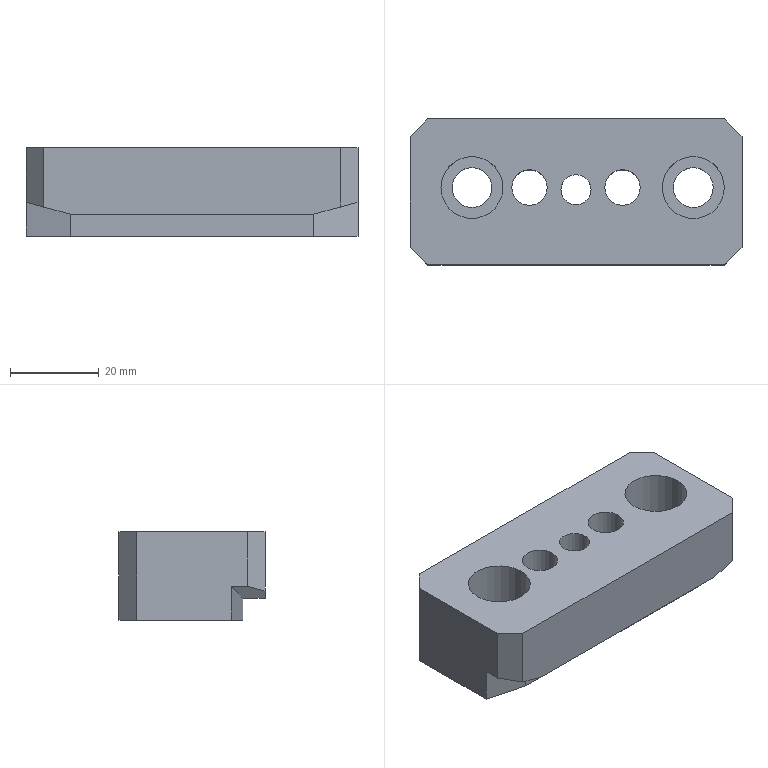Part | NX | features 20 2 | 1 solid | 25 faces | box 75 x 33 x 20 mm | volume 39698 mm3 | plane 18 | cylinder 7 | commonest cylinder face diameters 8.001 x2 9 x2 14 x2 6.8 x1
STEP:
#1=CARTESIAN_POINT('',(1899.002,435.,-3.5));
#2=VERTEX_POINT('',#1);
#3=CARTESIAN_POINT('',(1894.502,435.,-3.5));
#4=DIRECTION('',(0.,0.,-1.));
#5=DIRECTION('',(1.,0.,0.));
#6=AXIS2_PLACEMENT_3D('',#3,#4,#5);
#7=CIRCLE('',#6,4.5);
#8=EDGE_CURVE('',#2,#2,#7,.T.);
#9=ORIENTED_EDGE('',*,*,#8,.F.);
#10=EDGE_LOOP('',(#9));
#11=FACE_BOUND('',#10,.T.);
#12=CARTESIAN_POINT('',(1871.402,434.5,-3.5));
#13=VERTEX_POINT('',#12);
#14=CARTESIAN_POINT('',(1868.002,434.5,-3.5));
#15=DIRECTION('',(0.,0.,-1.));
#16=DIRECTION('',(1.,0.,0.));
#17=AXIS2_PLACEMENT_3D('',#14,#15,#16);
#18=CIRCLE('',#17,3.4);
#19=EDGE_CURVE('',#13,#13,#18,.T.);
#20=ORIENTED_EDGE('',*,*,#19,.F.);
#21=EDGE_LOOP('',(#20));
#22=FACE_BOUND('',#21,.T.);
#23=CARTESIAN_POINT('',(1849.002,435.,-3.5));
#24=VERTEX_POINT('',#23);
#25=CARTESIAN_POINT('',(1844.502,435.,-3.5));
#26=DIRECTION('',(0.,0.,1.));
#27=DIRECTION('',(1.,0.,0.));
#28=AXIS2_PLACEMENT_3D('',#25,#26,#27);
#29=CIRCLE('',#28,4.5);
#30=EDGE_CURVE('',#24,#24,#29,.T.);
#31=ORIENTED_EDGE('',*,*,#30,.T.);
#32=EDGE_LOOP('',(#31));
#33=FACE_BOUND('',#32,.T.);
#34=CARTESIAN_POINT('',(1895.501,422.5,-3.5));
#35=VERTEX_POINT('',#34);
#36=CARTESIAN_POINT('',(1840.501,422.5,-3.5));
#37=VERTEX_POINT('',#36);
#38=CARTESIAN_POINT('',(1906.501,422.5,-3.5));
#39=DIRECTION('',(-1.,0.,0.));
#40=VECTOR('',#39,1000.);
#41=LINE('',#38,#40);
#42=EDGE_CURVE('',#35,#37,#41,.T.);
#43=ORIENTED_EDGE('',*,*,#42,.T.);
#44=CARTESIAN_POINT('',(1830.502,425.179,-3.5));
#45=VERTEX_POINT('',#44);
#46=CARTESIAN_POINT('',(1840.501,422.5,-3.5));
#47=DIRECTION('',(-0.9659,0.2588,0.));
#48=VECTOR('',#47,1000.);
#49=LINE('',#46,#48);
#50=EDGE_CURVE('',#37,#45,#49,.T.);
#51=ORIENTED_EDGE('',*,*,#50,.T.);
#52=CARTESIAN_POINT('',(1830.502,446.5,-3.5));
#53=VERTEX_POINT('',#52);
#54=CARTESIAN_POINT('',(1830.502,417.5,-3.5));
#55=DIRECTION('',(0.,1.,0.));
#56=VECTOR('',#55,1000.);
#57=LINE('',#54,#56);
#58=EDGE_CURVE('',#45,#53,#57,.T.);
#59=ORIENTED_EDGE('',*,*,#58,.T.);
#60=CARTESIAN_POINT('',(1834.502,450.5,-3.5));
#61=VERTEX_POINT('',#60);
#62=CARTESIAN_POINT('',(1834.502,450.5,-3.5));
#63=DIRECTION('',(-0.7071,-0.7071,0.));
#64=VECTOR('',#63,1000.);
#65=LINE('',#62,#64);
#66=EDGE_CURVE('',#61,#53,#65,.T.);
#67=ORIENTED_EDGE('',*,*,#66,.F.);
#68=CARTESIAN_POINT('',(1901.502,450.5,-3.5));
#69=VERTEX_POINT('',#68);
#70=CARTESIAN_POINT('',(1948.502,450.5,-3.5));
#71=DIRECTION('',(1.,0.,0.));
#72=VECTOR('',#71,1000.);
#73=LINE('',#70,#72);
#74=EDGE_CURVE('',#61,#69,#73,.T.);
#75=ORIENTED_EDGE('',*,*,#74,.T.);
#76=CARTESIAN_POINT('',(1905.502,446.5,-3.5));
#77=VERTEX_POINT('',#76);
#78=CARTESIAN_POINT('',(1905.502,446.5,-3.5));
#79=DIRECTION('',(-0.7071,0.7071,0.));
#80=VECTOR('',#79,1000.);
#81=LINE('',#78,#80);
#82=EDGE_CURVE('',#77,#69,#81,.T.);
#83=ORIENTED_EDGE('',*,*,#82,.F.);
#84=CARTESIAN_POINT('',(1905.502,425.18,-3.5));
#85=VERTEX_POINT('',#84);
#86=CARTESIAN_POINT('',(1905.502,450.5,-3.5));
#87=DIRECTION('',(0.,-1.,0.));
#88=VECTOR('',#87,1000.);
#89=LINE('',#86,#88);
#90=EDGE_CURVE('',#77,#85,#89,.T.);
#91=ORIENTED_EDGE('',*,*,#90,.T.);
#92=CARTESIAN_POINT('',(1905.502,425.18,-3.5));
#93=DIRECTION('',(-0.9659,-0.2588,0.));
#94=VECTOR('',#93,1000.);
#95=LINE('',#92,#94);
#96=EDGE_CURVE('',#85,#35,#95,.T.);
#97=ORIENTED_EDGE('',*,*,#96,.T.);
#98=EDGE_LOOP('',(#43,#51,#59,#67,#75,#83,#91,#97));
#99=FACE_BOUND('',#98,.T.);
#100=CARTESIAN_POINT('',(1861.503,435.,-3.5));
#101=VERTEX_POINT('',#100);
#102=CARTESIAN_POINT('',(1857.502,435.,-3.5));
#103=DIRECTION('',(0.,0.,1.));
#104=DIRECTION('',(1.,0.,0.));
#105=AXIS2_PLACEMENT_3D('',#102,#103,#104);
#106=CIRCLE('',#105,4.);
#107=EDGE_CURVE('',#101,#101,#106,.T.);
#108=ORIENTED_EDGE('',*,*,#107,.T.);
#109=EDGE_LOOP('',(#108));
#110=FACE_BOUND('',#109,.T.);
#111=CARTESIAN_POINT('',(1882.503,435.,-3.5));
#112=VERTEX_POINT('',#111);
#113=CARTESIAN_POINT('',(1878.502,435.,-3.5));
#114=DIRECTION('',(0.,0.,-1.));
#115=DIRECTION('',(1.,0.,0.));
#116=AXIS2_PLACEMENT_3D('',#113,#114,#115);
#117=CIRCLE('',#116,4.);
#118=EDGE_CURVE('',#112,#112,#117,.T.);
#119=ORIENTED_EDGE('',*,*,#118,.F.);
#120=EDGE_LOOP('',(#119));
#121=FACE_BOUND('',#120,.T.);
#122=CARTESIAN_POINT('',(2018.502,450.5,-3.5));
#123=DIRECTION('',(0.,0.,1.));
#124=DIRECTION('',(-1.,0.,0.));
#125=AXIS2_PLACEMENT_3D('',#122,#123,#124);
#126=PLANE('',#125);
#127=ADVANCED_FACE('',(#11,#22,#33,#99,#110,#121),#126,.F.);
#128=CARTESIAN_POINT('',(1840.502,417.5,1.5));
#129=VERTEX_POINT('',#128);
#130=CARTESIAN_POINT('',(1895.502,417.5,1.5));
#131=VERTEX_POINT('',#130);
#132=CARTESIAN_POINT('',(1966.502,417.5,1.5));
#133=DIRECTION('',(1.,0.,0.));
#134=VECTOR('',#133,1000.);
#135=LINE('',#132,#134);
#136=EDGE_CURVE('',#129,#131,#135,.T.);
#137=ORIENTED_EDGE('',*,*,#136,.T.);
#138=CARTESIAN_POINT('',(1901.502,417.5,3.108));
#139=VERTEX_POINT('',#138);
#140=CARTESIAN_POINT('',(1895.502,417.5,1.5));
#141=DIRECTION('',(-0.9659,0.,-0.2588));
#142=VECTOR('',#141,1000.);
#143=LINE('',#140,#142);
#144=EDGE_CURVE('',#139,#131,#143,.T.);
#145=ORIENTED_EDGE('',*,*,#144,.F.);
#146=CARTESIAN_POINT('',(1901.502,417.5,16.5));
#147=VERTEX_POINT('',#146);
#148=CARTESIAN_POINT('',(1901.502,417.5,11.5));
#149=DIRECTION('',(0.,0.,-1.));
#150=VECTOR('',#149,1000.);
#151=LINE('',#148,#150);
#152=EDGE_CURVE('',#147,#139,#151,.T.);
#153=ORIENTED_EDGE('',*,*,#152,.F.);
#154=CARTESIAN_POINT('',(1834.502,417.5,16.5));
#155=VERTEX_POINT('',#154);
#156=CARTESIAN_POINT('',(1968.502,417.5,16.5));
#157=DIRECTION('',(-1.,0.,0.));
#158=VECTOR('',#157,1000.);
#159=LINE('',#156,#158);
#160=EDGE_CURVE('',#147,#155,#159,.T.);
#161=ORIENTED_EDGE('',*,*,#160,.T.);
#162=CARTESIAN_POINT('',(1834.502,417.5,3.108));
#163=VERTEX_POINT('',#162);
#164=CARTESIAN_POINT('',(1834.502,417.5,11.5));
#165=DIRECTION('',(0.,0.,1.));
#166=VECTOR('',#165,1000.);
#167=LINE('',#164,#166);
#168=EDGE_CURVE('',#163,#155,#167,.T.);
#169=ORIENTED_EDGE('',*,*,#168,.F.);
#170=CARTESIAN_POINT('',(1840.502,417.5,1.5));
#171=DIRECTION('',(-0.9659,0.,0.2588));
#172=VECTOR('',#171,1000.);
#173=LINE('',#170,#172);
#174=EDGE_CURVE('',#129,#163,#173,.T.);
#175=ORIENTED_EDGE('',*,*,#174,.F.);
#176=EDGE_LOOP('',(#137,#145,#153,#161,#169,#175));
#177=FACE_BOUND('',#176,.T.);
#178=CARTESIAN_POINT('',(1968.502,417.5,11.5));
#179=DIRECTION('',(0.,1.,0.));
#180=DIRECTION('',(0.,0.,1.));
#181=AXIS2_PLACEMENT_3D('',#178,#179,#180);
#182=PLANE('',#181);
#183=ADVANCED_FACE('',(#177),#182,.F.);
#184=CARTESIAN_POINT('',(1882.503,435.,16.5));
#185=VERTEX_POINT('',#184);
#186=CARTESIAN_POINT('',(1878.502,435.,16.5));
#187=DIRECTION('',(0.,0.,1.));
#188=DIRECTION('',(1.,0.,0.));
#189=AXIS2_PLACEMENT_3D('',#186,#187,#188);
#190=CIRCLE('',#189,4.);
#191=EDGE_CURVE('',#185,#185,#190,.T.);
#192=ORIENTED_EDGE('',*,*,#191,.F.);
#193=EDGE_LOOP('',(#192));
#194=FACE_BOUND('',#193,.T.);
#195=CARTESIAN_POINT('',(1861.503,435.,16.5));
#196=VERTEX_POINT('',#195);
#197=CARTESIAN_POINT('',(1857.502,435.,16.5));
#198=DIRECTION('',(0.,0.,1.));
#199=DIRECTION('',(1.,0.,0.));
#200=AXIS2_PLACEMENT_3D('',#197,#198,#199);
#201=CIRCLE('',#200,4.);
#202=EDGE_CURVE('',#196,#196,#201,.T.);
#203=ORIENTED_EDGE('',*,*,#202,.F.);
#204=EDGE_LOOP('',(#203));
#205=FACE_BOUND('',#204,.T.);
#206=CARTESIAN_POINT('',(1901.502,435.,16.5));
#207=VERTEX_POINT('',#206);
#208=CARTESIAN_POINT('',(1894.502,435.,16.5));
#209=DIRECTION('',(0.,0.,-1.));
#210=DIRECTION('',(1.,0.,0.));
#211=AXIS2_PLACEMENT_3D('',#208,#209,#210);
#212=CIRCLE('',#211,7.);
#213=EDGE_CURVE('',#207,#207,#212,.T.);
#214=ORIENTED_EDGE('',*,*,#213,.T.);
#215=EDGE_LOOP('',(#214));
#216=FACE_BOUND('',#215,.T.);
#217=CARTESIAN_POINT('',(1851.502,435.,16.5));
#218=VERTEX_POINT('',#217);
#219=CARTESIAN_POINT('',(1844.502,435.,16.5));
#220=DIRECTION('',(0.,0.,-1.));
#221=DIRECTION('',(1.,0.,0.));
#222=AXIS2_PLACEMENT_3D('',#219,#220,#221);
#223=CIRCLE('',#222,7.);
#224=EDGE_CURVE('',#218,#218,#223,.T.);
#225=ORIENTED_EDGE('',*,*,#224,.T.);
#226=EDGE_LOOP('',(#225));
#227=FACE_BOUND('',#226,.T.);
#228=ORIENTED_EDGE('',*,*,#160,.F.);
#229=CARTESIAN_POINT('',(1905.502,421.5,16.5));
#230=VERTEX_POINT('',#229);
#231=CARTESIAN_POINT('',(1901.502,417.5,16.5));
#232=DIRECTION('',(-0.7071,-0.7071,0.));
#233=VECTOR('',#232,1000.);
#234=LINE('',#231,#233);
#235=EDGE_CURVE('',#230,#147,#234,.T.);
#236=ORIENTED_EDGE('',*,*,#235,.F.);
#237=CARTESIAN_POINT('',(1905.502,446.5,16.5));
#238=VERTEX_POINT('',#237);
#239=CARTESIAN_POINT('',(1905.502,450.5,16.5));
#240=DIRECTION('',(0.,-1.,0.));
#241=VECTOR('',#240,1000.);
#242=LINE('',#239,#241);
#243=EDGE_CURVE('',#238,#230,#242,.T.);
#244=ORIENTED_EDGE('',*,*,#243,.F.);
#245=CARTESIAN_POINT('',(1901.502,450.5,16.5));
#246=VERTEX_POINT('',#245);
#247=CARTESIAN_POINT('',(1905.502,446.5,16.5));
#248=DIRECTION('',(0.7071,-0.7071,0.));
#249=VECTOR('',#248,1000.);
#250=LINE('',#247,#249);
#251=EDGE_CURVE('',#246,#238,#250,.T.);
#252=ORIENTED_EDGE('',*,*,#251,.F.);
#253=CARTESIAN_POINT('',(1834.502,450.5,16.5));
#254=VERTEX_POINT('',#253);
#255=CARTESIAN_POINT('',(1888.502,450.5,16.5));
#256=DIRECTION('',(1.,0.,0.));
#257=VECTOR('',#256,1000.);
#258=LINE('',#255,#257);
#259=EDGE_CURVE('',#254,#246,#258,.T.);
#260=ORIENTED_EDGE('',*,*,#259,.F.);
#261=CARTESIAN_POINT('',(1830.502,446.5,16.5));
#262=VERTEX_POINT('',#261);
#263=CARTESIAN_POINT('',(1834.502,450.5,16.5));
#264=DIRECTION('',(0.7071,0.7071,0.));
#265=VECTOR('',#264,1000.);
#266=LINE('',#263,#265);
#267=EDGE_CURVE('',#262,#254,#266,.T.);
#268=ORIENTED_EDGE('',*,*,#267,.F.);
#269=CARTESIAN_POINT('',(1830.502,421.5,16.5));
#270=VERTEX_POINT('',#269);
#271=CARTESIAN_POINT('',(1830.502,417.5,16.5));
#272=DIRECTION('',(0.,1.,0.));
#273=VECTOR('',#272,1000.);
#274=LINE('',#271,#273);
#275=EDGE_CURVE('',#270,#262,#274,.T.);
#276=ORIENTED_EDGE('',*,*,#275,.F.);
#277=CARTESIAN_POINT('',(1830.502,421.5,16.5));
#278=DIRECTION('',(-0.7071,0.7071,0.));
#279=VECTOR('',#278,1000.);
#280=LINE('',#277,#279);
#281=EDGE_CURVE('',#155,#270,#280,.T.);
#282=ORIENTED_EDGE('',*,*,#281,.F.);
#283=EDGE_LOOP('',(#228,#236,#244,#252,#260,#268,#276,#282));
#284=FACE_BOUND('',#283,.T.);
#285=CARTESIAN_POINT('',(1871.402,434.5,16.5));
#286=VERTEX_POINT('',#285);
#287=CARTESIAN_POINT('',(1868.002,434.5,16.5));
#288=DIRECTION('',(0.,0.,1.));
#289=DIRECTION('',(1.,0.,0.));
#290=AXIS2_PLACEMENT_3D('',#287,#288,#289);
#291=CIRCLE('',#290,3.4);
#292=EDGE_CURVE('',#286,#286,#291,.T.);
#293=ORIENTED_EDGE('',*,*,#292,.F.);
#294=EDGE_LOOP('',(#293));
#295=FACE_BOUND('',#294,.T.);
#296=CARTESIAN_POINT('',(1968.502,450.5,16.5));
#297=DIRECTION('',(0.,0.,1.));
#298=DIRECTION('',(-1.,0.,0.));
#299=AXIS2_PLACEMENT_3D('',#296,#297,#298);
#300=PLANE('',#299);
#301=ADVANCED_FACE('',(#194,#205,#216,#227,#284,#295),#300,.T.);
#302=CARTESIAN_POINT('',(1890.002,435.,6.5));
#303=VERTEX_POINT('',#302);
#304=CARTESIAN_POINT('',(1894.502,435.,6.5));
#305=DIRECTION('',(0.,0.,1.));
#306=DIRECTION('',(-1.,0.,0.));
#307=AXIS2_PLACEMENT_3D('',#304,#305,#306);
#308=CIRCLE('',#307,4.5);
#309=EDGE_CURVE('',#303,#303,#308,.T.);
#310=ORIENTED_EDGE('',*,*,#309,.F.);
#311=EDGE_LOOP('',(#310));
#312=FACE_BOUND('',#311,.T.);
#313=CARTESIAN_POINT('',(1887.502,435.,6.5));
#314=VERTEX_POINT('',#313);
#315=CARTESIAN_POINT('',(1894.502,435.,6.5));
#316=DIRECTION('',(0.,0.,-1.));
#317=DIRECTION('',(-1.,0.,0.));
#318=AXIS2_PLACEMENT_3D('',#315,#316,#317);
#319=CIRCLE('',#318,7.);
#320=EDGE_CURVE('',#314,#314,#319,.T.);
#321=ORIENTED_EDGE('',*,*,#320,.F.);
#322=EDGE_LOOP('',(#321));
#323=FACE_BOUND('',#322,.T.);
#324=CARTESIAN_POINT('',(1894.502,432.5,6.5));
#325=DIRECTION('',(0.,0.,-1.));
#326=DIRECTION('',(1.,0.,0.));
#327=AXIS2_PLACEMENT_3D('',#324,#325,#326);
#328=PLANE('',#327);
#329=ADVANCED_FACE('',(#312,#323),#328,.F.);
#330=CARTESIAN_POINT('',(1895.502,422.5,1.5));
#331=VERTEX_POINT('',#330);
#332=CARTESIAN_POINT('',(1895.502,425.18,1.5));
#333=DIRECTION('',(0.,1.,0.));
#334=VECTOR('',#333,1000.);
#335=LINE('',#332,#334);
#336=EDGE_CURVE('',#131,#331,#335,.T.);
#337=ORIENTED_EDGE('',*,*,#336,.T.);
#338=CARTESIAN_POINT('',(1905.502,425.18,4.179));
#339=VERTEX_POINT('',#338);
#340=CARTESIAN_POINT('',(1904.875,425.012,4.011));
#341=DIRECTION('',(0.9351,0.2506,0.2506));
#342=VECTOR('',#341,1000.);
#343=LINE('',#340,#342);
#344=EDGE_CURVE('',#331,#339,#343,.T.);
#345=ORIENTED_EDGE('',*,*,#344,.T.);
#346=CARTESIAN_POINT('',(1905.502,421.5,4.179));
#347=VERTEX_POINT('',#346);
#348=CARTESIAN_POINT('',(1905.502,417.5,4.179));
#349=DIRECTION('',(0.,-1.,0.));
#350=VECTOR('',#349,1000.);
#351=LINE('',#348,#350);
#352=EDGE_CURVE('',#339,#347,#351,.T.);
#353=ORIENTED_EDGE('',*,*,#352,.T.);
#354=CARTESIAN_POINT('',(1888.451,404.449,-0.3894));
#355=DIRECTION('',(0.6947,0.6947,0.1862));
#356=VECTOR('',#355,1000.);
#357=LINE('',#354,#356);
#358=EDGE_CURVE('',#139,#347,#357,.T.);
#359=ORIENTED_EDGE('',*,*,#358,.F.);
#360=ORIENTED_EDGE('',*,*,#144,.T.);
#361=EDGE_LOOP('',(#337,#345,#353,#359,#360));
#362=FACE_BOUND('',#361,.T.);
#363=CARTESIAN_POINT('',(1895.502,396.891,1.5));
#364=DIRECTION('',(0.2588,0.,-0.9659));
#365=DIRECTION('',(0.9659,0.,0.2588));
#366=AXIS2_PLACEMENT_3D('',#363,#364,#365);
#367=PLANE('',#366);
#368=ADVANCED_FACE('',(#362),#367,.T.);
#369=CARTESIAN_POINT('',(1840.002,435.,6.5));
#370=VERTEX_POINT('',#369);
#371=CARTESIAN_POINT('',(1844.502,435.,6.5));
#372=DIRECTION('',(0.,0.,1.));
#373=DIRECTION('',(-1.,0.,0.));
#374=AXIS2_PLACEMENT_3D('',#371,#372,#373);
#375=CIRCLE('',#374,4.5);
#376=EDGE_CURVE('',#370,#370,#375,.T.);
#377=ORIENTED_EDGE('',*,*,#376,.F.);
#378=EDGE_LOOP('',(#377));
#379=FACE_BOUND('',#378,.T.);
#380=CARTESIAN_POINT('',(1837.502,435.,6.5));
#381=VERTEX_POINT('',#380);
#382=CARTESIAN_POINT('',(1844.502,435.,6.5));
#383=DIRECTION('',(0.,0.,-1.));
#384=DIRECTION('',(-1.,0.,0.));
#385=AXIS2_PLACEMENT_3D('',#382,#383,#384);
#386=CIRCLE('',#385,7.);
#387=EDGE_CURVE('',#381,#381,#386,.T.);
#388=ORIENTED_EDGE('',*,*,#387,.F.);
#389=EDGE_LOOP('',(#388));
#390=FACE_BOUND('',#389,.T.);
#391=CARTESIAN_POINT('',(1844.502,432.5,6.5));
#392=DIRECTION('',(0.,0.,-1.));
#393=DIRECTION('',(-1.,0.,0.));
#394=AXIS2_PLACEMENT_3D('',#391,#392,#393);
#395=PLANE('',#394);
#396=ADVANCED_FACE('',(#379,#390),#395,.F.);
#397=ORIENTED_EDGE('',*,*,#213,.F.);
#398=EDGE_LOOP('',(#397));
#399=FACE_BOUND('',#398,.T.);
#400=ORIENTED_EDGE('',*,*,#320,.T.);
#401=EDGE_LOOP('',(#400));
#402=FACE_BOUND('',#401,.T.);
#403=CARTESIAN_POINT('',(1894.502,435.,42.5));
#404=DIRECTION('',(0.,0.,-1.));
#405=DIRECTION('',(1.,0.,0.));
#406=AXIS2_PLACEMENT_3D('',#403,#404,#405);
#407=CYLINDRICAL_SURFACE('',#406,7.);
#408=ADVANCED_FACE('',(#399,#402),#407,.F.);
#409=ORIENTED_EDGE('',*,*,#235,.T.);
#410=ORIENTED_EDGE('',*,*,#152,.T.);
#411=ORIENTED_EDGE('',*,*,#358,.T.);
#412=CARTESIAN_POINT('',(1905.502,421.5,11.5));
#413=DIRECTION('',(0.,0.,1.));
#414=VECTOR('',#413,1000.);
#415=LINE('',#412,#414);
#416=EDGE_CURVE('',#347,#230,#415,.T.);
#417=ORIENTED_EDGE('',*,*,#416,.T.);
#418=EDGE_LOOP('',(#409,#410,#411,#417));
#419=FACE_BOUND('',#418,.T.);
#420=CARTESIAN_POINT('',(1901.502,417.5,11.5));
#421=DIRECTION('',(-0.7071,0.7071,0.));
#422=DIRECTION('',(0.,0.,-1.));
#423=AXIS2_PLACEMENT_3D('',#420,#421,#422);
#424=PLANE('',#423);
#425=ADVANCED_FACE('',(#419),#424,.F.);
#426=ORIENTED_EDGE('',*,*,#387,.T.);
#427=EDGE_LOOP('',(#426));
#428=FACE_BOUND('',#427,.T.);
#429=ORIENTED_EDGE('',*,*,#224,.F.);
#430=EDGE_LOOP('',(#429));
#431=FACE_BOUND('',#430,.T.);
#432=CARTESIAN_POINT('',(1844.502,435.,42.5));
#433=DIRECTION('',(0.,0.,-1.));
#434=DIRECTION('',(-1.,0.,0.));
#435=AXIS2_PLACEMENT_3D('',#432,#433,#434);
#436=CYLINDRICAL_SURFACE('',#435,7.);
#437=ADVANCED_FACE('',(#428,#431),#436,.F.);
#438=ORIENTED_EDGE('',*,*,#352,.F.);
#439=CARTESIAN_POINT('',(1905.502,425.18,3.5));
#440=DIRECTION('',(0.,0.,-1.));
#441=VECTOR('',#440,1000.);
#442=LINE('',#439,#441);
#443=EDGE_CURVE('',#339,#85,#442,.T.);
#444=ORIENTED_EDGE('',*,*,#443,.T.);
#445=ORIENTED_EDGE('',*,*,#90,.F.);
#446=CARTESIAN_POINT('',(1905.502,446.5,11.5));
#447=DIRECTION('',(0.,0.,-1.));
#448=VECTOR('',#447,1000.);
#449=LINE('',#446,#448);
#450=EDGE_CURVE('',#238,#77,#449,.T.);
#451=ORIENTED_EDGE('',*,*,#450,.F.);
#452=ORIENTED_EDGE('',*,*,#243,.T.);
#453=ORIENTED_EDGE('',*,*,#416,.F.);
#454=EDGE_LOOP('',(#438,#444,#445,#451,#452,#453));
#455=FACE_BOUND('',#454,.T.);
#456=CARTESIAN_POINT('',(1905.502,450.5,11.5));
#457=DIRECTION('',(-1.,0.,0.));
#458=DIRECTION('',(0.,0.,-1.));
#459=AXIS2_PLACEMENT_3D('',#456,#457,#458);
#460=PLANE('',#459);
#461=ADVANCED_FACE('',(#455),#460,.F.);
#462=CARTESIAN_POINT('',(1895.501,422.5,1.5));
#463=VERTEX_POINT('',#462);
#464=CARTESIAN_POINT('',(1905.502,425.18,1.5));
#465=DIRECTION('',(0.9659,0.2588,0.));
#466=VECTOR('',#465,1000.);
#467=LINE('',#464,#466);
#468=EDGE_CURVE('',#463,#331,#467,.T.);
#469=ORIENTED_EDGE('',*,*,#468,.F.);
#470=CARTESIAN_POINT('',(1895.501,422.5,3.5));
#471=DIRECTION('',(0.,0.,1.));
#472=VECTOR('',#471,1000.);
#473=LINE('',#470,#472);
#474=EDGE_CURVE('',#35,#463,#473,.T.);
#475=ORIENTED_EDGE('',*,*,#474,.F.);
#476=ORIENTED_EDGE('',*,*,#96,.F.);
#477=ORIENTED_EDGE('',*,*,#443,.F.);
#478=ORIENTED_EDGE('',*,*,#344,.F.);
#479=EDGE_LOOP('',(#469,#475,#476,#477,#478));
#480=FACE_BOUND('',#479,.T.);
#481=CARTESIAN_POINT('',(1905.502,425.18,3.5));
#482=DIRECTION('',(-0.2588,0.9659,0.));
#483=DIRECTION('',(0.9659,0.2588,0.));
#484=AXIS2_PLACEMENT_3D('',#481,#482,#483);
#485=PLANE('',#484);
#486=ADVANCED_FACE('',(#480),#485,.F.);
#487=ORIENTED_EDGE('',*,*,#309,.T.);
#488=EDGE_LOOP('',(#487));
#489=FACE_BOUND('',#488,.T.);
#490=ORIENTED_EDGE('',*,*,#8,.T.);
#491=EDGE_LOOP('',(#490));
#492=FACE_BOUND('',#491,.T.);
#493=CARTESIAN_POINT('',(1894.502,435.,42.5));
#494=DIRECTION('',(0.,0.,-1.));
#495=DIRECTION('',(1.,0.,0.));
#496=AXIS2_PLACEMENT_3D('',#493,#494,#495);
#497=CYLINDRICAL_SURFACE('',#496,4.5);
#498=ADVANCED_FACE('',(#489,#492),#497,.F.);
#499=CARTESIAN_POINT('',(1830.502,421.5,4.179));
#500=VERTEX_POINT('',#499);
#501=CARTESIAN_POINT('',(1830.502,421.5,11.5));
#502=DIRECTION('',(0.,0.,-1.));
#503=VECTOR('',#502,1000.);
#504=LINE('',#501,#503);
#505=EDGE_CURVE('',#270,#500,#504,.T.);
#506=ORIENTED_EDGE('',*,*,#505,.T.);
#507=CARTESIAN_POINT('',(1847.554,404.449,-0.3894));
#508=DIRECTION('',(0.6947,-0.6947,-0.1862));
#509=VECTOR('',#508,1000.);
#510=LINE('',#507,#509);
#511=EDGE_CURVE('',#500,#163,#510,.T.);
#512=ORIENTED_EDGE('',*,*,#511,.T.);
#513=ORIENTED_EDGE('',*,*,#168,.T.);
#514=ORIENTED_EDGE('',*,*,#281,.T.);
#515=EDGE_LOOP('',(#506,#512,#513,#514));
#516=FACE_BOUND('',#515,.T.);
#517=CARTESIAN_POINT('',(1830.502,421.5,11.5));
#518=DIRECTION('',(0.7071,0.7071,0.));
#519=DIRECTION('',(0.,0.,-1.));
#520=AXIS2_PLACEMENT_3D('',#517,#518,#519);
#521=PLANE('',#520);
#522=ADVANCED_FACE('',(#516),#521,.F.);
#523=ORIENTED_EDGE('',*,*,#30,.F.);
#524=EDGE_LOOP('',(#523));
#525=FACE_BOUND('',#524,.T.);
#526=ORIENTED_EDGE('',*,*,#376,.T.);
#527=EDGE_LOOP('',(#526));
#528=FACE_BOUND('',#527,.T.);
#529=CARTESIAN_POINT('',(1844.502,435.,42.5));
#530=DIRECTION('',(0.,0.,-1.));
#531=DIRECTION('',(-1.,0.,0.));
#532=AXIS2_PLACEMENT_3D('',#529,#530,#531);
#533=CYLINDRICAL_SURFACE('',#532,4.5);
#534=ADVANCED_FACE('',(#525,#528),#533,.F.);
#535=ORIENTED_EDGE('',*,*,#58,.F.);
#536=CARTESIAN_POINT('',(1830.502,425.179,4.179));
#537=VERTEX_POINT('',#536);
#538=CARTESIAN_POINT('',(1830.502,425.179,3.5));
#539=DIRECTION('',(0.,0.,-1.));
#540=VECTOR('',#539,1000.);
#541=LINE('',#538,#540);
#542=EDGE_CURVE('',#537,#45,#541,.T.);
#543=ORIENTED_EDGE('',*,*,#542,.F.);
#544=CARTESIAN_POINT('',(1830.502,425.179,4.179));
#545=DIRECTION('',(0.,1.,0.));
#546=VECTOR('',#545,1000.);
#547=LINE('',#544,#546);
#548=EDGE_CURVE('',#500,#537,#547,.T.);
#549=ORIENTED_EDGE('',*,*,#548,.F.);
#550=ORIENTED_EDGE('',*,*,#505,.F.);
#551=ORIENTED_EDGE('',*,*,#275,.T.);
#552=CARTESIAN_POINT('',(1830.502,446.5,11.5));
#553=DIRECTION('',(0.,0.,1.));
#554=VECTOR('',#553,1000.);
#555=LINE('',#552,#554);
#556=EDGE_CURVE('',#53,#262,#555,.T.);
#557=ORIENTED_EDGE('',*,*,#556,.F.);
#558=EDGE_LOOP('',(#535,#543,#549,#550,#551,#557));
#559=FACE_BOUND('',#558,.T.);
#560=CARTESIAN_POINT('',(1830.502,417.5,11.5));
#561=DIRECTION('',(1.,0.,0.));
#562=DIRECTION('',(0.,0.,1.));
#563=AXIS2_PLACEMENT_3D('',#560,#561,#562);
#564=PLANE('',#563);
#565=ADVANCED_FACE('',(#559),#564,.F.);
#566=ORIENTED_EDGE('',*,*,#548,.T.);
#567=CARTESIAN_POINT('',(1840.501,422.5,1.5));
#568=VERTEX_POINT('',#567);
#569=CARTESIAN_POINT('',(1840.501,422.5,1.5));
#570=DIRECTION('',(0.9351,-0.2506,-0.2506));
#571=VECTOR('',#570,1000.);
#572=LINE('',#569,#571);
#573=EDGE_CURVE('',#537,#568,#572,.T.);
#574=ORIENTED_EDGE('',*,*,#573,.T.);
#575=CARTESIAN_POINT('',(1840.502,422.5,1.5));
#576=VERTEX_POINT('',#575);
#577=CARTESIAN_POINT('',(1840.502,422.5,1.5));
#578=DIRECTION('',(0.9659,0.,-0.2588));
#579=VECTOR('',#578,1000.);
#580=LINE('',#577,#579);
#581=EDGE_CURVE('',#568,#576,#580,.T.);
#582=ORIENTED_EDGE('',*,*,#581,.T.);
#583=CARTESIAN_POINT('',(1840.502,417.5,1.5));
#584=DIRECTION('',(0.,-1.,0.));
#585=VECTOR('',#584,1000.);
#586=LINE('',#583,#585);
#587=EDGE_CURVE('',#576,#129,#586,.T.);
#588=ORIENTED_EDGE('',*,*,#587,.T.);
#589=ORIENTED_EDGE('',*,*,#174,.T.);
#590=ORIENTED_EDGE('',*,*,#511,.F.);
#591=EDGE_LOOP('',(#566,#574,#582,#588,#589,#590));
#592=FACE_BOUND('',#591,.T.);
#593=CARTESIAN_POINT('',(1840.502,396.891,1.5));
#594=DIRECTION('',(-0.2588,0.,-0.9659));
#595=DIRECTION('',(0.9659,0.,-0.2588));
#596=AXIS2_PLACEMENT_3D('',#593,#594,#595);
#597=PLANE('',#596);
#598=ADVANCED_FACE('',(#592),#597,.T.);
#599=ORIENTED_EDGE('',*,*,#50,.F.);
#600=CARTESIAN_POINT('',(1840.501,422.5,3.5));
#601=DIRECTION('',(0.,0.,1.));
#602=VECTOR('',#601,1000.);
#603=LINE('',#600,#602);
#604=EDGE_CURVE('',#37,#568,#603,.T.);
#605=ORIENTED_EDGE('',*,*,#604,.T.);
#606=ORIENTED_EDGE('',*,*,#573,.F.);
#607=ORIENTED_EDGE('',*,*,#542,.T.);
#608=EDGE_LOOP('',(#599,#605,#606,#607));
#609=FACE_BOUND('',#608,.T.);
#610=CARTESIAN_POINT('',(1840.501,422.5,3.5));
#611=DIRECTION('',(0.2588,0.9659,0.));
#612=DIRECTION('',(0.9659,-0.2588,0.));
#613=AXIS2_PLACEMENT_3D('',#610,#611,#612);
#614=PLANE('',#613);
#615=ADVANCED_FACE('',(#609),#614,.F.);
#616=ORIENTED_EDGE('',*,*,#66,.T.);
#617=ORIENTED_EDGE('',*,*,#556,.T.);
#618=ORIENTED_EDGE('',*,*,#267,.T.);
#619=CARTESIAN_POINT('',(1834.502,450.5,11.5));
#620=DIRECTION('',(0.,0.,-1.));
#621=VECTOR('',#620,1000.);
#622=LINE('',#619,#621);
#623=EDGE_CURVE('',#254,#61,#622,.T.);
#624=ORIENTED_EDGE('',*,*,#623,.T.);
#625=EDGE_LOOP('',(#616,#617,#618,#624));
#626=FACE_BOUND('',#625,.T.);
#627=CARTESIAN_POINT('',(1834.502,450.5,11.5));
#628=DIRECTION('',(0.7071,-0.7071,0.));
#629=DIRECTION('',(0.,0.,-1.));
#630=AXIS2_PLACEMENT_3D('',#627,#628,#629);
#631=PLANE('',#630);
#632=ADVANCED_FACE('',(#626),#631,.F.);
#633=ORIENTED_EDGE('',*,*,#82,.T.);
#634=CARTESIAN_POINT('',(1901.502,450.5,11.5));
#635=DIRECTION('',(0.,0.,1.));
#636=VECTOR('',#635,1000.);
#637=LINE('',#634,#636);
#638=EDGE_CURVE('',#69,#246,#637,.T.);
#639=ORIENTED_EDGE('',*,*,#638,.T.);
#640=ORIENTED_EDGE('',*,*,#251,.T.);
#641=ORIENTED_EDGE('',*,*,#450,.T.);
#642=EDGE_LOOP('',(#633,#639,#640,#641));
#643=FACE_BOUND('',#642,.T.);
#644=CARTESIAN_POINT('',(1905.502,446.5,11.5));
#645=DIRECTION('',(-0.7071,-0.7071,0.));
#646=DIRECTION('',(0.,0.,-1.));
#647=AXIS2_PLACEMENT_3D('',#644,#645,#646);
#648=PLANE('',#647);
#649=ADVANCED_FACE('',(#643),#648,.F.);
#650=ORIENTED_EDGE('',*,*,#638,.F.);
#651=ORIENTED_EDGE('',*,*,#74,.F.);
#652=ORIENTED_EDGE('',*,*,#623,.F.);
#653=ORIENTED_EDGE('',*,*,#259,.T.);
#654=EDGE_LOOP('',(#650,#651,#652,#653));
#655=FACE_BOUND('',#654,.T.);
#656=CARTESIAN_POINT('',(1888.502,450.5,11.5));
#657=DIRECTION('',(0.,-1.,0.));
#658=DIRECTION('',(0.,0.,-1.));
#659=AXIS2_PLACEMENT_3D('',#656,#657,#658);
#660=PLANE('',#659);
#661=ADVANCED_FACE('',(#655),#660,.F.);
#662=CARTESIAN_POINT('',(1956.501,422.5,1.5));
#663=DIRECTION('',(1.,0.,0.));
#664=VECTOR('',#663,1000.);
#665=LINE('',#662,#664);
#666=EDGE_CURVE('',#576,#463,#665,.T.);
#667=ORIENTED_EDGE('',*,*,#666,.T.);
#668=ORIENTED_EDGE('',*,*,#468,.T.);
#669=ORIENTED_EDGE('',*,*,#336,.F.);
#670=ORIENTED_EDGE('',*,*,#136,.F.);
#671=ORIENTED_EDGE('',*,*,#587,.F.);
#672=EDGE_LOOP('',(#667,#668,#669,#670,#671));
#673=FACE_BOUND('',#672,.T.);
#674=CARTESIAN_POINT('',(1988.773,396.891,1.5));
#675=DIRECTION('',(0.,0.,-1.));
#676=DIRECTION('',(1.,0.,0.));
#677=AXIS2_PLACEMENT_3D('',#674,#675,#676);
#678=PLANE('',#677);
#679=ADVANCED_FACE('',(#673),#678,.T.);
#680=ORIENTED_EDGE('',*,*,#474,.T.);
#681=ORIENTED_EDGE('',*,*,#666,.F.);
#682=ORIENTED_EDGE('',*,*,#581,.F.);
#683=ORIENTED_EDGE('',*,*,#604,.F.);
#684=ORIENTED_EDGE('',*,*,#42,.F.);
#685=EDGE_LOOP('',(#680,#681,#682,#683,#684));
#686=FACE_BOUND('',#685,.T.);
#687=CARTESIAN_POINT('',(1906.501,422.5,3.5));
#688=DIRECTION('',(0.,1.,0.));
#689=DIRECTION('',(0.,0.,1.));
#690=AXIS2_PLACEMENT_3D('',#687,#688,#689);
#691=PLANE('',#690);
#692=ADVANCED_FACE('',(#686),#691,.F.);
#693=ORIENTED_EDGE('',*,*,#292,.T.);
#694=EDGE_LOOP('',(#693));
#695=FACE_BOUND('',#694,.T.);
#696=ORIENTED_EDGE('',*,*,#19,.T.);
#697=EDGE_LOOP('',(#696));
#698=FACE_BOUND('',#697,.T.);
#699=CARTESIAN_POINT('',(1868.002,434.5,16.5));
#700=DIRECTION('',(0.,0.,-1.));
#701=DIRECTION('',(-1.,0.,0.));
#702=AXIS2_PLACEMENT_3D('',#699,#700,#701);
#703=CYLINDRICAL_SURFACE('',#702,3.4);
#704=ADVANCED_FACE('',(#695,#698),#703,.F.);
#705=ORIENTED_EDGE('',*,*,#202,.T.);
#706=EDGE_LOOP('',(#705));
#707=FACE_BOUND('',#706,.T.);
#708=ORIENTED_EDGE('',*,*,#107,.F.);
#709=EDGE_LOOP('',(#708));
#710=FACE_BOUND('',#709,.T.);
#711=CARTESIAN_POINT('',(1857.502,435.,-3.5));
#712=DIRECTION('',(0.,0.,1.));
#713=DIRECTION('',(-1.,0.,0.));
#714=AXIS2_PLACEMENT_3D('',#711,#712,#713);
#715=CYLINDRICAL_SURFACE('',#714,4.);
#716=ADVANCED_FACE('',(#707,#710),#715,.F.);
#717=ORIENTED_EDGE('',*,*,#191,.T.);
#718=EDGE_LOOP('',(#717));
#719=FACE_BOUND('',#718,.T.);
#720=ORIENTED_EDGE('',*,*,#118,.T.);
#721=EDGE_LOOP('',(#720));
#722=FACE_BOUND('',#721,.T.);
#723=CARTESIAN_POINT('',(1878.502,435.,-3.5));
#724=DIRECTION('',(0.,0.,1.));
#725=DIRECTION('',(1.,0.,0.));
#726=AXIS2_PLACEMENT_3D('',#723,#724,#725);
#727=CYLINDRICAL_SURFACE('',#726,4.);
#728=ADVANCED_FACE('',(#719,#722),#727,.F.);
#729=CLOSED_SHELL('',(#127,#183,#301,#329,#368,#396,#408,#425,#437,#461,#486,#498,#522,#534,#565,#598,#615,#632,#649,#661,#679,#692,#704,#716,#728));
#730=MANIFOLD_SOLID_BREP('',#729);
#731=(LENGTH_UNIT()NAMED_UNIT(*)SI_UNIT(.MILLI.,.METRE.));
#732=UNCERTAINTY_MEASURE_WITH_UNIT(LENGTH_MEASURE(0.00001),#731,'','');
#733=(NAMED_UNIT(*)PLANE_ANGLE_UNIT()SI_UNIT($,.RADIAN.));
#734=(NAMED_UNIT(*)SI_UNIT($,.STERADIAN.)SOLID_ANGLE_UNIT());
#735=(GEOMETRIC_REPRESENTATION_CONTEXT(3)GLOBAL_UNCERTAINTY_ASSIGNED_CONTEXT((#732))GLOBAL_UNIT_ASSIGNED_CONTEXT((#731,#733,#734))REPRESENTATION_CONTEXT('',''));
#736=ADVANCED_BREP_SHAPE_REPRESENTATION('',(#730),#735);